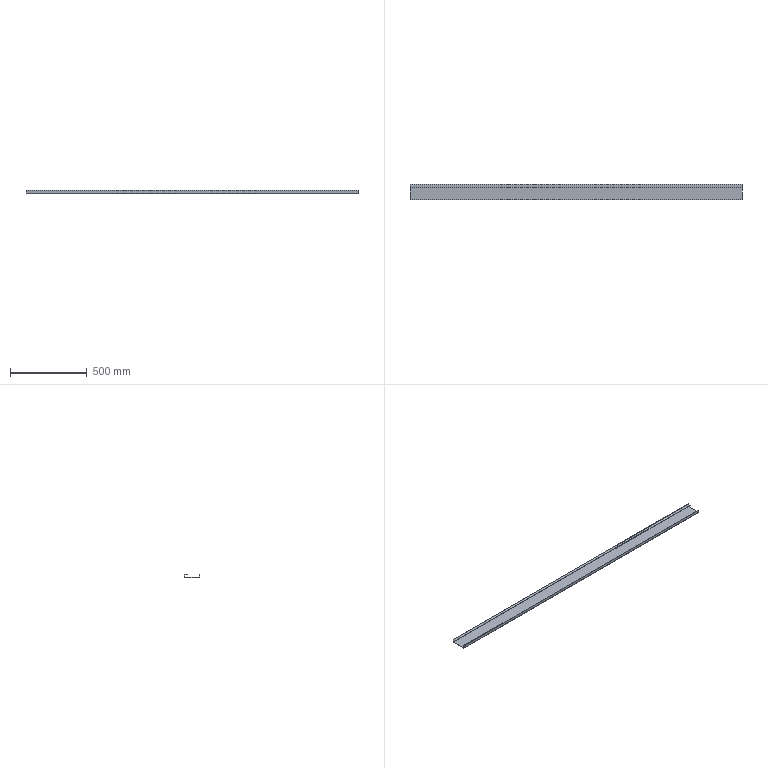Part | STEP file | 粉仓踢脚Plate 5 | 1 solid | 18 faces | box 2168 x 100 x 20 mm | volume 498243 mm3 | plane 12 | cylinder 6 | commonest cylinder face diameters 2 x3 5 x3
STEP:
#1=CARTESIAN_POINT('',(0.,0.,0.));
#2=DIRECTION('',(0.,0.,1.));
#3=DIRECTION('',(1.,0.,0.));
#4=AXIS2_PLACEMENT_3D('',#1,#2,#3);
#5=CARTESIAN_POINT('',(-1083.75,1.5,2.5));
#6=VERTEX_POINT('',#5);
#7=CARTESIAN_POINT('',(-1083.75,1.5,20.));
#8=VERTEX_POINT('',#7);
#9=CARTESIAN_POINT('',(-1083.75,1.5,2.5));
#10=DIRECTION('',(0.,0.,1.));
#11=VECTOR('',#10,1.);
#12=LINE('',#9,#11);
#13=CARTESIAN_POINT('',(1083.75,1.5,2.5));
#14=DIRECTION('',(0.,-1.,0.));
#15=DIRECTION('',(0.,0.,-1.));
#16=AXIS2_PLACEMENT_3D('',#13,#14,#15);
#17=PLANE('',#16);
#18=CARTESIAN_POINT('',(0.,-2167.5));
#19=DIRECTION('',(-1.,0.));
#20=VECTOR('',#19,1.);
#21=LINE('',#18,#20);
#22=(GEOMETRIC_REPRESENTATION_CONTEXT(2)PARAMETRIC_REPRESENTATION_CONTEXT()REPRESENTATION_CONTEXT('',''));
#23=DEFINITIONAL_REPRESENTATION('',(#21),#22);
#24=PCURVE('',#17,#23);
#25=CARTESIAN_POINT('',(-1083.75,2.5,2.5));
#26=DIRECTION('',(-1.,0.,0.));
#27=DIRECTION('',(0.,0.,1.));
#28=AXIS2_PLACEMENT_3D('',#25,#26,#27);
#29=PLANE('',#28);
#30=CARTESIAN_POINT('',(0.,-1.));
#31=DIRECTION('',(1.,0.));
#32=VECTOR('',#31,1.);
#33=LINE('',#30,#32);
#34=(GEOMETRIC_REPRESENTATION_CONTEXT(2)PARAMETRIC_REPRESENTATION_CONTEXT()REPRESENTATION_CONTEXT('',''));
#35=DEFINITIONAL_REPRESENTATION('',(#33),#34);
#36=PCURVE('',#29,#35);
#37=SURFACE_CURVE('',#12,(#24,#36),.PCURVE_S1.);
#38=EDGE_CURVE('',#6,#8,#37,.T.);
#39=ORIENTED_EDGE('',*,*,#38,.T.);
#40=CARTESIAN_POINT('',(1083.75,1.5,20.));
#41=VERTEX_POINT('',#40);
#42=CARTESIAN_POINT('',(1083.75,1.5,20.));
#43=DIRECTION('',(-1.,0.,0.));
#44=VECTOR('',#43,1.);
#45=LINE('',#42,#44);
#46=CARTESIAN_POINT('',(-17.5,0.));
#47=DIRECTION('',(0.,-1.));
#48=VECTOR('',#47,1.);
#49=LINE('',#46,#48);
#50=(GEOMETRIC_REPRESENTATION_CONTEXT(2)PARAMETRIC_REPRESENTATION_CONTEXT()REPRESENTATION_CONTEXT('',''));
#51=DEFINITIONAL_REPRESENTATION('',(#49),#50);
#52=PCURVE('',#17,#51);
#53=CARTESIAN_POINT('',(1083.75,0.,20.));
#54=DIRECTION('',(0.,0.,1.));
#55=DIRECTION('',(1.,0.,0.));
#56=AXIS2_PLACEMENT_3D('',#53,#54,#55);
#57=PLANE('',#56);
#58=CARTESIAN_POINT('',(0.,1.5));
#59=DIRECTION('',(-1.,0.));
#60=VECTOR('',#59,1.);
#61=LINE('',#58,#60);
#62=(GEOMETRIC_REPRESENTATION_CONTEXT(2)PARAMETRIC_REPRESENTATION_CONTEXT()REPRESENTATION_CONTEXT('',''));
#63=DEFINITIONAL_REPRESENTATION('',(#61),#62);
#64=PCURVE('',#57,#63);
#65=SURFACE_CURVE('',#45,(#52,#64),.PCURVE_S1.);
#66=EDGE_CURVE('',#41,#8,#65,.T.);
#67=ORIENTED_EDGE('',*,*,#66,.F.);
#68=CARTESIAN_POINT('',(1083.75,1.5,2.5));
#69=VERTEX_POINT('',#68);
#70=CARTESIAN_POINT('',(1083.75,1.5,2.5));
#71=DIRECTION('',(0.,0.,1.));
#72=VECTOR('',#71,1.);
#73=LINE('',#70,#72);
#74=CARTESIAN_POINT('',(0.,0.));
#75=DIRECTION('',(-1.,0.));
#76=VECTOR('',#75,1.);
#77=LINE('',#74,#76);
#78=(GEOMETRIC_REPRESENTATION_CONTEXT(2)PARAMETRIC_REPRESENTATION_CONTEXT()REPRESENTATION_CONTEXT('',''));
#79=DEFINITIONAL_REPRESENTATION('',(#77),#78);
#80=PCURVE('',#17,#79);
#81=CARTESIAN_POINT('',(1083.75,2.5,2.5));
#82=DIRECTION('',(-1.,0.,0.));
#83=DIRECTION('',(0.,0.,1.));
#84=AXIS2_PLACEMENT_3D('',#81,#82,#83);
#85=PLANE('',#84);
#86=CARTESIAN_POINT('',(0.,-1.));
#87=DIRECTION('',(1.,0.));
#88=VECTOR('',#87,1.);
#89=LINE('',#86,#88);
#90=(GEOMETRIC_REPRESENTATION_CONTEXT(2)PARAMETRIC_REPRESENTATION_CONTEXT()REPRESENTATION_CONTEXT('',''));
#91=DEFINITIONAL_REPRESENTATION('',(#89),#90);
#92=PCURVE('',#85,#91);
#93=SURFACE_CURVE('',#73,(#80,#92),.PCURVE_S1.);
#94=EDGE_CURVE('',#69,#41,#93,.T.);
#95=ORIENTED_EDGE('',*,*,#94,.F.);
#96=CARTESIAN_POINT('',(1083.75,1.5,2.5));
#97=DIRECTION('',(-1.,0.,0.));
#98=VECTOR('',#97,1.);
#99=LINE('',#96,#98);
#100=CARTESIAN_POINT('',(0.,0.));
#101=DIRECTION('',(0.,-1.));
#102=VECTOR('',#101,1.);
#103=LINE('',#100,#102);
#104=(GEOMETRIC_REPRESENTATION_CONTEXT(2)PARAMETRIC_REPRESENTATION_CONTEXT()REPRESENTATION_CONTEXT('',''));
#105=DEFINITIONAL_REPRESENTATION('',(#103),#104);
#106=PCURVE('',#17,#105);
#107=CARTESIAN_POINT('',(1083.75,2.5,2.5));
#108=DIRECTION('',(-1.,0.,0.));
#109=DIRECTION('',(0.,0.,1.));
#110=AXIS2_PLACEMENT_3D('',#107,#108,#109);
#111=CYLINDRICAL_SURFACE('',#110,1.);
#112=CARTESIAN_POINT('',(4.712,0.));
#113=DIRECTION('',(0.,1.));
#114=VECTOR('',#113,1.);
#115=LINE('',#112,#114);
#116=(GEOMETRIC_REPRESENTATION_CONTEXT(2)PARAMETRIC_REPRESENTATION_CONTEXT()REPRESENTATION_CONTEXT('',''));
#117=DEFINITIONAL_REPRESENTATION('',(#115),#116);
#118=PCURVE('',#111,#117);
#119=SURFACE_CURVE('',#99,(#106,#118),.PCURVE_S1.);
#120=EDGE_CURVE('',#69,#6,#119,.T.);
#121=ORIENTED_EDGE('',*,*,#120,.T.);
#122=EDGE_LOOP('',(#39,#67,#95,#121));
#123=FACE_BOUND('',#122,.T.);
#124=ADVANCED_FACE('',(#123),#17,.F.);
#125=CARTESIAN_POINT('',(-1083.75,0.,20.));
#126=VERTEX_POINT('',#125);
#127=CARTESIAN_POINT('',(-1083.75,0.,20.));
#128=DIRECTION('',(0.,1.,0.));
#129=VECTOR('',#128,1.);
#130=LINE('',#127,#129);
#131=CARTESIAN_POINT('',(-2167.5,0.));
#132=DIRECTION('',(0.,1.));
#133=VECTOR('',#132,1.);
#134=LINE('',#131,#133);
#135=(GEOMETRIC_REPRESENTATION_CONTEXT(2)PARAMETRIC_REPRESENTATION_CONTEXT()REPRESENTATION_CONTEXT('',''));
#136=DEFINITIONAL_REPRESENTATION('',(#134),#135);
#137=PCURVE('',#57,#136);
#138=CARTESIAN_POINT('',(17.5,-2.5));
#139=DIRECTION('',(0.,1.));
#140=VECTOR('',#139,1.);
#141=LINE('',#138,#140);
#142=(GEOMETRIC_REPRESENTATION_CONTEXT(2)PARAMETRIC_REPRESENTATION_CONTEXT()REPRESENTATION_CONTEXT('',''));
#143=DEFINITIONAL_REPRESENTATION('',(#141),#142);
#144=PCURVE('',#29,#143);
#145=SURFACE_CURVE('',#130,(#137,#144),.PCURVE_S1.);
#146=EDGE_CURVE('',#126,#8,#145,.T.);
#147=ORIENTED_EDGE('',*,*,#146,.F.);
#148=CARTESIAN_POINT('',(1083.75,0.,20.));
#149=VERTEX_POINT('',#148);
#150=CARTESIAN_POINT('',(1083.75,0.,20.));
#151=DIRECTION('',(-1.,0.,0.));
#152=VECTOR('',#151,1.);
#153=LINE('',#150,#152);
#154=CARTESIAN_POINT('',(0.,0.));
#155=DIRECTION('',(-1.,0.));
#156=VECTOR('',#155,1.);
#157=LINE('',#154,#156);
#158=(GEOMETRIC_REPRESENTATION_CONTEXT(2)PARAMETRIC_REPRESENTATION_CONTEXT()REPRESENTATION_CONTEXT('',''));
#159=DEFINITIONAL_REPRESENTATION('',(#157),#158);
#160=PCURVE('',#57,#159);
#161=CARTESIAN_POINT('',(1083.75,0.,2.5));
#162=DIRECTION('',(0.,-1.,0.));
#163=DIRECTION('',(0.,0.,-1.));
#164=AXIS2_PLACEMENT_3D('',#161,#162,#163);
#165=PLANE('',#164);
#166=CARTESIAN_POINT('',(-17.5,0.));
#167=DIRECTION('',(0.,-1.));
#168=VECTOR('',#167,1.);
#169=LINE('',#166,#168);
#170=(GEOMETRIC_REPRESENTATION_CONTEXT(2)PARAMETRIC_REPRESENTATION_CONTEXT()REPRESENTATION_CONTEXT('',''));
#171=DEFINITIONAL_REPRESENTATION('',(#169),#170);
#172=PCURVE('',#165,#171);
#173=SURFACE_CURVE('',#153,(#160,#172),.PCURVE_S1.);
#174=EDGE_CURVE('',#149,#126,#173,.T.);
#175=ORIENTED_EDGE('',*,*,#174,.F.);
#176=CARTESIAN_POINT('',(1083.75,0.,20.));
#177=DIRECTION('',(0.,1.,0.));
#178=VECTOR('',#177,1.);
#179=LINE('',#176,#178);
#180=CARTESIAN_POINT('',(0.,0.));
#181=DIRECTION('',(0.,1.));
#182=VECTOR('',#181,1.);
#183=LINE('',#180,#182);
#184=(GEOMETRIC_REPRESENTATION_CONTEXT(2)PARAMETRIC_REPRESENTATION_CONTEXT()REPRESENTATION_CONTEXT('',''));
#185=DEFINITIONAL_REPRESENTATION('',(#183),#184);
#186=PCURVE('',#57,#185);
#187=CARTESIAN_POINT('',(17.5,-2.5));
#188=DIRECTION('',(0.,1.));
#189=VECTOR('',#188,1.);
#190=LINE('',#187,#189);
#191=(GEOMETRIC_REPRESENTATION_CONTEXT(2)PARAMETRIC_REPRESENTATION_CONTEXT()REPRESENTATION_CONTEXT('',''));
#192=DEFINITIONAL_REPRESENTATION('',(#190),#191);
#193=PCURVE('',#85,#192);
#194=SURFACE_CURVE('',#179,(#186,#193),.PCURVE_S1.);
#195=EDGE_CURVE('',#149,#41,#194,.T.);
#196=ORIENTED_EDGE('',*,*,#195,.T.);
#197=ORIENTED_EDGE('',*,*,#66,.T.);
#198=EDGE_LOOP('',(#147,#175,#196,#197));
#199=FACE_BOUND('',#198,.T.);
#200=ADVANCED_FACE('',(#199),#57,.T.);
#201=CARTESIAN_POINT('',(-1083.75,0.,2.5));
#202=VERTEX_POINT('',#201);
#203=CARTESIAN_POINT('',(-1083.75,0.,2.5));
#204=DIRECTION('',(0.,0.,1.));
#205=VECTOR('',#204,1.);
#206=LINE('',#203,#205);
#207=CARTESIAN_POINT('',(0.,-2167.5));
#208=DIRECTION('',(-1.,0.));
#209=VECTOR('',#208,1.);
#210=LINE('',#207,#209);
#211=(GEOMETRIC_REPRESENTATION_CONTEXT(2)PARAMETRIC_REPRESENTATION_CONTEXT()REPRESENTATION_CONTEXT('',''));
#212=DEFINITIONAL_REPRESENTATION('',(#210),#211);
#213=PCURVE('',#165,#212);
#214=CARTESIAN_POINT('',(0.,-2.5));
#215=DIRECTION('',(1.,0.));
#216=VECTOR('',#215,1.);
#217=LINE('',#214,#216);
#218=(GEOMETRIC_REPRESENTATION_CONTEXT(2)PARAMETRIC_REPRESENTATION_CONTEXT()REPRESENTATION_CONTEXT('',''));
#219=DEFINITIONAL_REPRESENTATION('',(#217),#218);
#220=PCURVE('',#29,#219);
#221=SURFACE_CURVE('',#206,(#213,#220),.PCURVE_S1.);
#222=EDGE_CURVE('',#202,#126,#221,.T.);
#223=ORIENTED_EDGE('',*,*,#222,.F.);
#224=CARTESIAN_POINT('',(1083.75,0.,2.5));
#225=VERTEX_POINT('',#224);
#226=CARTESIAN_POINT('',(1083.75,0.,2.5));
#227=DIRECTION('',(-1.,0.,0.));
#228=VECTOR('',#227,1.);
#229=LINE('',#226,#228);
#230=CARTESIAN_POINT('',(0.,0.));
#231=DIRECTION('',(0.,-1.));
#232=VECTOR('',#231,1.);
#233=LINE('',#230,#232);
#234=(GEOMETRIC_REPRESENTATION_CONTEXT(2)PARAMETRIC_REPRESENTATION_CONTEXT()REPRESENTATION_CONTEXT('',''));
#235=DEFINITIONAL_REPRESENTATION('',(#233),#234);
#236=PCURVE('',#165,#235);
#237=CARTESIAN_POINT('',(1083.75,2.5,2.5));
#238=DIRECTION('',(-1.,0.,0.));
#239=DIRECTION('',(0.,0.,1.));
#240=AXIS2_PLACEMENT_3D('',#237,#238,#239);
#241=CYLINDRICAL_SURFACE('',#240,2.5);
#242=CARTESIAN_POINT('',(4.712,0.));
#243=DIRECTION('',(0.,1.));
#244=VECTOR('',#243,1.);
#245=LINE('',#242,#244);
#246=(GEOMETRIC_REPRESENTATION_CONTEXT(2)PARAMETRIC_REPRESENTATION_CONTEXT()REPRESENTATION_CONTEXT('',''));
#247=DEFINITIONAL_REPRESENTATION('',(#245),#246);
#248=PCURVE('',#241,#247);
#249=SURFACE_CURVE('',#229,(#236,#248),.PCURVE_S1.);
#250=EDGE_CURVE('',#225,#202,#249,.T.);
#251=ORIENTED_EDGE('',*,*,#250,.F.);
#252=CARTESIAN_POINT('',(1083.75,0.,2.5));
#253=DIRECTION('',(0.,0.,1.));
#254=VECTOR('',#253,1.);
#255=LINE('',#252,#254);
#256=CARTESIAN_POINT('',(0.,0.));
#257=DIRECTION('',(-1.,0.));
#258=VECTOR('',#257,1.);
#259=LINE('',#256,#258);
#260=(GEOMETRIC_REPRESENTATION_CONTEXT(2)PARAMETRIC_REPRESENTATION_CONTEXT()REPRESENTATION_CONTEXT('',''));
#261=DEFINITIONAL_REPRESENTATION('',(#259),#260);
#262=PCURVE('',#165,#261);
#263=CARTESIAN_POINT('',(0.,-2.5));
#264=DIRECTION('',(1.,0.));
#265=VECTOR('',#264,1.);
#266=LINE('',#263,#265);
#267=(GEOMETRIC_REPRESENTATION_CONTEXT(2)PARAMETRIC_REPRESENTATION_CONTEXT()REPRESENTATION_CONTEXT('',''));
#268=DEFINITIONAL_REPRESENTATION('',(#266),#267);
#269=PCURVE('',#85,#268);
#270=SURFACE_CURVE('',#255,(#262,#269),.PCURVE_S1.);
#271=EDGE_CURVE('',#225,#149,#270,.T.);
#272=ORIENTED_EDGE('',*,*,#271,.T.);
#273=ORIENTED_EDGE('',*,*,#174,.T.);
#274=EDGE_LOOP('',(#223,#251,#272,#273));
#275=FACE_BOUND('',#274,.T.);
#276=ADVANCED_FACE('',(#275),#165,.T.);
#277=CARTESIAN_POINT('',(-1083.75,2.5,0.));
#278=VERTEX_POINT('',#277);
#279=CARTESIAN_POINT('',(-1083.75,2.5,2.5));
#280=DIRECTION('',(-1.,0.,0.));
#281=DIRECTION('',(0.,0.,1.));
#282=AXIS2_PLACEMENT_3D('',#279,#280,#281);
#283=CIRCLE('',#282,2.5);
#284=CARTESIAN_POINT('',(0.,2167.5));
#285=DIRECTION('',(1.,0.));
#286=VECTOR('',#285,1.);
#287=LINE('',#284,#286);
#288=(GEOMETRIC_REPRESENTATION_CONTEXT(2)PARAMETRIC_REPRESENTATION_CONTEXT()REPRESENTATION_CONTEXT('',''));
#289=DEFINITIONAL_REPRESENTATION('',(#287),#288);
#290=PCURVE('',#241,#289);
#291=CARTESIAN_POINT('',(0.,0.));
#292=DIRECTION('',(1.,0.));
#293=AXIS2_PLACEMENT_2D('',#291,#292);
#294=CIRCLE('',#293,2.5);
#295=(GEOMETRIC_REPRESENTATION_CONTEXT(2)PARAMETRIC_REPRESENTATION_CONTEXT()REPRESENTATION_CONTEXT('',''));
#296=DEFINITIONAL_REPRESENTATION('',(#294),#295);
#297=PCURVE('',#29,#296);
#298=SURFACE_CURVE('',#283,(#290,#297),.PCURVE_S1.);
#299=EDGE_CURVE('',#278,#202,#298,.T.);
#300=ORIENTED_EDGE('',*,*,#299,.F.);
#301=CARTESIAN_POINT('',(1083.75,2.5,0.));
#302=VERTEX_POINT('',#301);
#303=CARTESIAN_POINT('',(1083.75,2.5,0.));
#304=DIRECTION('',(-1.,0.,0.));
#305=VECTOR('',#304,1.);
#306=LINE('',#303,#305);
#307=CARTESIAN_POINT('',(3.142,0.));
#308=DIRECTION('',(0.,1.));
#309=VECTOR('',#308,1.);
#310=LINE('',#307,#309);
#311=(GEOMETRIC_REPRESENTATION_CONTEXT(2)PARAMETRIC_REPRESENTATION_CONTEXT()REPRESENTATION_CONTEXT('',''));
#312=DEFINITIONAL_REPRESENTATION('',(#310),#311);
#313=PCURVE('',#241,#312);
#314=CARTESIAN_POINT('',(1083.75,2.5,0.));
#315=DIRECTION('',(0.,0.,-1.));
#316=DIRECTION('',(-1.,0.,0.));
#317=AXIS2_PLACEMENT_3D('',#314,#315,#316);
#318=PLANE('',#317);
#319=CARTESIAN_POINT('',(0.,0.));
#320=DIRECTION('',(1.,0.));
#321=VECTOR('',#320,1.);
#322=LINE('',#319,#321);
#323=(GEOMETRIC_REPRESENTATION_CONTEXT(2)PARAMETRIC_REPRESENTATION_CONTEXT()REPRESENTATION_CONTEXT('',''));
#324=DEFINITIONAL_REPRESENTATION('',(#322),#323);
#325=PCURVE('',#318,#324);
#326=SURFACE_CURVE('',#306,(#313,#325),.PCURVE_S1.);
#327=EDGE_CURVE('',#302,#278,#326,.T.);
#328=ORIENTED_EDGE('',*,*,#327,.F.);
#329=CARTESIAN_POINT('',(1083.75,2.5,2.5));
#330=DIRECTION('',(-1.,0.,0.));
#331=DIRECTION('',(0.,0.,1.));
#332=AXIS2_PLACEMENT_3D('',#329,#330,#331);
#333=CIRCLE('',#332,2.5);
#334=CARTESIAN_POINT('',(0.,0.));
#335=DIRECTION('',(1.,0.));
#336=VECTOR('',#335,1.);
#337=LINE('',#334,#336);
#338=(GEOMETRIC_REPRESENTATION_CONTEXT(2)PARAMETRIC_REPRESENTATION_CONTEXT()REPRESENTATION_CONTEXT('',''));
#339=DEFINITIONAL_REPRESENTATION('',(#337),#338);
#340=PCURVE('',#241,#339);
#341=CARTESIAN_POINT('',(0.,0.));
#342=DIRECTION('',(1.,0.));
#343=AXIS2_PLACEMENT_2D('',#341,#342);
#344=CIRCLE('',#343,2.5);
#345=(GEOMETRIC_REPRESENTATION_CONTEXT(2)PARAMETRIC_REPRESENTATION_CONTEXT()REPRESENTATION_CONTEXT('',''));
#346=DEFINITIONAL_REPRESENTATION('',(#344),#345);
#347=PCURVE('',#85,#346);
#348=SURFACE_CURVE('',#333,(#340,#347),.PCURVE_S1.);
#349=EDGE_CURVE('',#302,#225,#348,.T.);
#350=ORIENTED_EDGE('',*,*,#349,.T.);
#351=ORIENTED_EDGE('',*,*,#250,.T.);
#352=EDGE_LOOP('',(#300,#328,#350,#351));
#353=FACE_BOUND('',#352,.T.);
#354=ADVANCED_FACE('',(#353),#241,.T.);
#355=CARTESIAN_POINT('',(-1083.75,97.5,0.));
#356=VERTEX_POINT('',#355);
#357=CARTESIAN_POINT('',(-1083.75,2.5,0.));
#358=DIRECTION('',(0.,-1.,0.));
#359=VECTOR('',#358,1.);
#360=LINE('',#357,#359);
#361=CARTESIAN_POINT('',(2167.5,0.));
#362=DIRECTION('',(0.,-1.));
#363=VECTOR('',#362,1.);
#364=LINE('',#361,#363);
#365=(GEOMETRIC_REPRESENTATION_CONTEXT(2)PARAMETRIC_REPRESENTATION_CONTEXT()REPRESENTATION_CONTEXT('',''));
#366=DEFINITIONAL_REPRESENTATION('',(#364),#365);
#367=PCURVE('',#318,#366);
#368=CARTESIAN_POINT('',(-2.5,0.));
#369=DIRECTION('',(0.,-1.));
#370=VECTOR('',#369,1.);
#371=LINE('',#368,#370);
#372=(GEOMETRIC_REPRESENTATION_CONTEXT(2)PARAMETRIC_REPRESENTATION_CONTEXT()REPRESENTATION_CONTEXT('',''));
#373=DEFINITIONAL_REPRESENTATION('',(#371),#372);
#374=PCURVE('',#29,#373);
#375=SURFACE_CURVE('',#360,(#367,#374),.PCURVE_S1.);
#376=EDGE_CURVE('',#356,#278,#375,.T.);
#377=ORIENTED_EDGE('',*,*,#376,.F.);
#378=CARTESIAN_POINT('',(1083.75,97.5,0.));
#379=VERTEX_POINT('',#378);
#380=CARTESIAN_POINT('',(1083.75,97.5,0.));
#381=DIRECTION('',(-1.,0.,0.));
#382=VECTOR('',#381,1.);
#383=LINE('',#380,#382);
#384=CARTESIAN_POINT('',(0.,95.));
#385=DIRECTION('',(1.,0.));
#386=VECTOR('',#385,1.);
#387=LINE('',#384,#386);
#388=(GEOMETRIC_REPRESENTATION_CONTEXT(2)PARAMETRIC_REPRESENTATION_CONTEXT()REPRESENTATION_CONTEXT('',''));
#389=DEFINITIONAL_REPRESENTATION('',(#387),#388);
#390=PCURVE('',#318,#389);
#391=CARTESIAN_POINT('',(1083.75,97.5,2.5));
#392=DIRECTION('',(-1.,0.,0.));
#393=DIRECTION('',(0.,0.,1.));
#394=AXIS2_PLACEMENT_3D('',#391,#392,#393);
#395=CYLINDRICAL_SURFACE('',#394,2.5);
#396=CARTESIAN_POINT('',(3.142,0.));
#397=DIRECTION('',(0.,1.));
#398=VECTOR('',#397,1.);
#399=LINE('',#396,#398);
#400=(GEOMETRIC_REPRESENTATION_CONTEXT(2)PARAMETRIC_REPRESENTATION_CONTEXT()REPRESENTATION_CONTEXT('',''));
#401=DEFINITIONAL_REPRESENTATION('',(#399),#400);
#402=PCURVE('',#395,#401);
#403=SURFACE_CURVE('',#383,(#390,#402),.PCURVE_S1.);
#404=EDGE_CURVE('',#379,#356,#403,.T.);
#405=ORIENTED_EDGE('',*,*,#404,.F.);
#406=CARTESIAN_POINT('',(1083.75,2.5,0.));
#407=DIRECTION('',(0.,-1.,0.));
#408=VECTOR('',#407,1.);
#409=LINE('',#406,#408);
#410=CARTESIAN_POINT('',(0.,0.));
#411=DIRECTION('',(0.,-1.));
#412=VECTOR('',#411,1.);
#413=LINE('',#410,#412);
#414=(GEOMETRIC_REPRESENTATION_CONTEXT(2)PARAMETRIC_REPRESENTATION_CONTEXT()REPRESENTATION_CONTEXT('',''));
#415=DEFINITIONAL_REPRESENTATION('',(#413),#414);
#416=PCURVE('',#318,#415);
#417=CARTESIAN_POINT('',(-2.5,0.));
#418=DIRECTION('',(0.,-1.));
#419=VECTOR('',#418,1.);
#420=LINE('',#417,#419);
#421=(GEOMETRIC_REPRESENTATION_CONTEXT(2)PARAMETRIC_REPRESENTATION_CONTEXT()REPRESENTATION_CONTEXT('',''));
#422=DEFINITIONAL_REPRESENTATION('',(#420),#421);
#423=PCURVE('',#85,#422);
#424=SURFACE_CURVE('',#409,(#416,#423),.PCURVE_S1.);
#425=EDGE_CURVE('',#379,#302,#424,.T.);
#426=ORIENTED_EDGE('',*,*,#425,.T.);
#427=ORIENTED_EDGE('',*,*,#327,.T.);
#428=EDGE_LOOP('',(#377,#405,#426,#427));
#429=FACE_BOUND('',#428,.T.);
#430=ADVANCED_FACE('',(#429),#318,.T.);
#431=CARTESIAN_POINT('',(-1083.75,100.,2.5));
#432=VERTEX_POINT('',#431);
#433=CARTESIAN_POINT('',(-1083.75,97.5,2.5));
#434=DIRECTION('',(-1.,0.,0.));
#435=DIRECTION('',(0.,0.,-1.));
#436=AXIS2_PLACEMENT_3D('',#433,#434,#435);
#437=CIRCLE('',#436,2.5);
#438=CARTESIAN_POINT('',(-3.142,2167.5));
#439=DIRECTION('',(1.,0.));
#440=VECTOR('',#439,1.);
#441=LINE('',#438,#440);
#442=(GEOMETRIC_REPRESENTATION_CONTEXT(2)PARAMETRIC_REPRESENTATION_CONTEXT()REPRESENTATION_CONTEXT('',''));
#443=DEFINITIONAL_REPRESENTATION('',(#441),#442);
#444=PCURVE('',#395,#443);
#445=CARTESIAN_POINT('',(0.,95.));
#446=DIRECTION('',(-1.,0.));
#447=AXIS2_PLACEMENT_2D('',#445,#446);
#448=CIRCLE('',#447,2.5);
#449=(GEOMETRIC_REPRESENTATION_CONTEXT(2)PARAMETRIC_REPRESENTATION_CONTEXT()REPRESENTATION_CONTEXT('',''));
#450=DEFINITIONAL_REPRESENTATION('',(#448),#449);
#451=PCURVE('',#29,#450);
#452=SURFACE_CURVE('',#437,(#444,#451),.PCURVE_S1.);
#453=EDGE_CURVE('',#432,#356,#452,.T.);
#454=ORIENTED_EDGE('',*,*,#453,.F.);
#455=CARTESIAN_POINT('',(1083.75,100.,2.5));
#456=VERTEX_POINT('',#455);
#457=CARTESIAN_POINT('',(1083.75,100.,2.5));
#458=DIRECTION('',(-1.,0.,0.));
#459=VECTOR('',#458,1.);
#460=LINE('',#457,#459);
#461=CARTESIAN_POINT('',(1.571,0.));
#462=DIRECTION('',(0.,1.));
#463=VECTOR('',#462,1.);
#464=LINE('',#461,#463);
#465=(GEOMETRIC_REPRESENTATION_CONTEXT(2)PARAMETRIC_REPRESENTATION_CONTEXT()REPRESENTATION_CONTEXT('',''));
#466=DEFINITIONAL_REPRESENTATION('',(#464),#465);
#467=PCURVE('',#395,#466);
#468=CARTESIAN_POINT('',(1083.75,100.,2.5));
#469=DIRECTION('',(0.,1.,0.));
#470=DIRECTION('',(0.,0.,1.));
#471=AXIS2_PLACEMENT_3D('',#468,#469,#470);
#472=PLANE('',#471);
#473=CARTESIAN_POINT('',(0.,0.));
#474=DIRECTION('',(0.,-1.));
#475=VECTOR('',#474,1.);
#476=LINE('',#473,#475);
#477=(GEOMETRIC_REPRESENTATION_CONTEXT(2)PARAMETRIC_REPRESENTATION_CONTEXT()REPRESENTATION_CONTEXT('',''));
#478=DEFINITIONAL_REPRESENTATION('',(#476),#477);
#479=PCURVE('',#472,#478);
#480=SURFACE_CURVE('',#460,(#467,#479),.PCURVE_S1.);
#481=EDGE_CURVE('',#456,#432,#480,.T.);
#482=ORIENTED_EDGE('',*,*,#481,.F.);
#483=CARTESIAN_POINT('',(1083.75,97.5,2.5));
#484=DIRECTION('',(-1.,0.,0.));
#485=DIRECTION('',(0.,0.,-1.));
#486=AXIS2_PLACEMENT_3D('',#483,#484,#485);
#487=CIRCLE('',#486,2.5);
#488=CARTESIAN_POINT('',(-3.142,0.));
#489=DIRECTION('',(1.,0.));
#490=VECTOR('',#489,1.);
#491=LINE('',#488,#490);
#492=(GEOMETRIC_REPRESENTATION_CONTEXT(2)PARAMETRIC_REPRESENTATION_CONTEXT()REPRESENTATION_CONTEXT('',''));
#493=DEFINITIONAL_REPRESENTATION('',(#491),#492);
#494=PCURVE('',#395,#493);
#495=CARTESIAN_POINT('',(0.,95.));
#496=DIRECTION('',(-1.,0.));
#497=AXIS2_PLACEMENT_2D('',#495,#496);
#498=CIRCLE('',#497,2.5);
#499=(GEOMETRIC_REPRESENTATION_CONTEXT(2)PARAMETRIC_REPRESENTATION_CONTEXT()REPRESENTATION_CONTEXT('',''));
#500=DEFINITIONAL_REPRESENTATION('',(#498),#499);
#501=PCURVE('',#85,#500);
#502=SURFACE_CURVE('',#487,(#494,#501),.PCURVE_S1.);
#503=EDGE_CURVE('',#456,#379,#502,.T.);
#504=ORIENTED_EDGE('',*,*,#503,.T.);
#505=ORIENTED_EDGE('',*,*,#404,.T.);
#506=EDGE_LOOP('',(#454,#482,#504,#505));
#507=FACE_BOUND('',#506,.T.);
#508=ADVANCED_FACE('',(#507),#395,.T.);
#509=CARTESIAN_POINT('',(-1083.75,100.,17.5));
#510=VERTEX_POINT('',#509);
#511=CARTESIAN_POINT('',(-1083.75,100.,2.5));
#512=DIRECTION('',(0.,0.,-1.));
#513=VECTOR('',#512,1.);
#514=LINE('',#511,#513);
#515=CARTESIAN_POINT('',(0.,-2167.5));
#516=DIRECTION('',(-1.,0.));
#517=VECTOR('',#516,1.);
#518=LINE('',#515,#517);
#519=(GEOMETRIC_REPRESENTATION_CONTEXT(2)PARAMETRIC_REPRESENTATION_CONTEXT()REPRESENTATION_CONTEXT('',''));
#520=DEFINITIONAL_REPRESENTATION('',(#518),#519);
#521=PCURVE('',#472,#520);
#522=CARTESIAN_POINT('',(0.,97.5));
#523=DIRECTION('',(-1.,0.));
#524=VECTOR('',#523,1.);
#525=LINE('',#522,#524);
#526=(GEOMETRIC_REPRESENTATION_CONTEXT(2)PARAMETRIC_REPRESENTATION_CONTEXT()REPRESENTATION_CONTEXT('',''));
#527=DEFINITIONAL_REPRESENTATION('',(#525),#526);
#528=PCURVE('',#29,#527);
#529=SURFACE_CURVE('',#514,(#521,#528),.PCURVE_S1.);
#530=EDGE_CURVE('',#510,#432,#529,.T.);
#531=ORIENTED_EDGE('',*,*,#530,.F.);
#532=CARTESIAN_POINT('',(1083.75,100.,17.5));
#533=VERTEX_POINT('',#532);
#534=CARTESIAN_POINT('',(1083.75,100.,17.5));
#535=DIRECTION('',(-1.,0.,0.));
#536=VECTOR('',#535,1.);
#537=LINE('',#534,#536);
#538=CARTESIAN_POINT('',(15.,0.));
#539=DIRECTION('',(0.,-1.));
#540=VECTOR('',#539,1.);
#541=LINE('',#538,#540);
#542=(GEOMETRIC_REPRESENTATION_CONTEXT(2)PARAMETRIC_REPRESENTATION_CONTEXT()REPRESENTATION_CONTEXT('',''));
#543=DEFINITIONAL_REPRESENTATION('',(#541),#542);
#544=PCURVE('',#472,#543);
#545=CARTESIAN_POINT('',(1083.75,97.5,17.5));
#546=DIRECTION('',(-1.,0.,0.));
#547=DIRECTION('',(0.,0.,1.));
#548=AXIS2_PLACEMENT_3D('',#545,#546,#547);
#549=CYLINDRICAL_SURFACE('',#548,2.5);
#550=CARTESIAN_POINT('',(1.571,0.));
#551=DIRECTION('',(0.,1.));
#552=VECTOR('',#551,1.);
#553=LINE('',#550,#552);
#554=(GEOMETRIC_REPRESENTATION_CONTEXT(2)PARAMETRIC_REPRESENTATION_CONTEXT()REPRESENTATION_CONTEXT('',''));
#555=DEFINITIONAL_REPRESENTATION('',(#553),#554);
#556=PCURVE('',#549,#555);
#557=SURFACE_CURVE('',#537,(#544,#556),.PCURVE_S1.);
#558=EDGE_CURVE('',#533,#510,#557,.T.);
#559=ORIENTED_EDGE('',*,*,#558,.F.);
#560=CARTESIAN_POINT('',(1083.75,100.,2.5));
#561=DIRECTION('',(0.,0.,-1.));
#562=VECTOR('',#561,1.);
#563=LINE('',#560,#562);
#564=CARTESIAN_POINT('',(0.,0.));
#565=DIRECTION('',(-1.,0.));
#566=VECTOR('',#565,1.);
#567=LINE('',#564,#566);
#568=(GEOMETRIC_REPRESENTATION_CONTEXT(2)PARAMETRIC_REPRESENTATION_CONTEXT()REPRESENTATION_CONTEXT('',''));
#569=DEFINITIONAL_REPRESENTATION('',(#567),#568);
#570=PCURVE('',#472,#569);
#571=CARTESIAN_POINT('',(0.,97.5));
#572=DIRECTION('',(-1.,0.));
#573=VECTOR('',#572,1.);
#574=LINE('',#571,#573);
#575=(GEOMETRIC_REPRESENTATION_CONTEXT(2)PARAMETRIC_REPRESENTATION_CONTEXT()REPRESENTATION_CONTEXT('',''));
#576=DEFINITIONAL_REPRESENTATION('',(#574),#575);
#577=PCURVE('',#85,#576);
#578=SURFACE_CURVE('',#563,(#570,#577),.PCURVE_S1.);
#579=EDGE_CURVE('',#533,#456,#578,.T.);
#580=ORIENTED_EDGE('',*,*,#579,.T.);
#581=ORIENTED_EDGE('',*,*,#481,.T.);
#582=EDGE_LOOP('',(#531,#559,#580,#581));
#583=FACE_BOUND('',#582,.T.);
#584=ADVANCED_FACE('',(#583),#472,.T.);
#585=CARTESIAN_POINT('',(-1083.75,97.5,20.));
#586=VERTEX_POINT('',#585);
#587=CARTESIAN_POINT('',(-1083.75,97.5,17.5));
#588=DIRECTION('',(-1.,0.,0.));
#589=DIRECTION('',(0.,0.,-1.));
#590=AXIS2_PLACEMENT_3D('',#587,#588,#589);
#591=CIRCLE('',#590,2.5);
#592=CARTESIAN_POINT('',(-3.142,2167.5));
#593=DIRECTION('',(1.,0.));
#594=VECTOR('',#593,1.);
#595=LINE('',#592,#594);
#596=(GEOMETRIC_REPRESENTATION_CONTEXT(2)PARAMETRIC_REPRESENTATION_CONTEXT()REPRESENTATION_CONTEXT('',''));
#597=DEFINITIONAL_REPRESENTATION('',(#595),#596);
#598=PCURVE('',#549,#597);
#599=CARTESIAN_POINT('',(15.,95.));
#600=DIRECTION('',(-1.,0.));
#601=AXIS2_PLACEMENT_2D('',#599,#600);
#602=CIRCLE('',#601,2.5);
#603=(GEOMETRIC_REPRESENTATION_CONTEXT(2)PARAMETRIC_REPRESENTATION_CONTEXT()REPRESENTATION_CONTEXT('',''));
#604=DEFINITIONAL_REPRESENTATION('',(#602),#603);
#605=PCURVE('',#29,#604);
#606=SURFACE_CURVE('',#591,(#598,#605),.PCURVE_S1.);
#607=EDGE_CURVE('',#586,#510,#606,.T.);
#608=ORIENTED_EDGE('',*,*,#607,.F.);
#609=CARTESIAN_POINT('',(1083.75,97.5,20.));
#610=VERTEX_POINT('',#609);
#611=CARTESIAN_POINT('',(1083.75,97.5,20.));
#612=DIRECTION('',(-1.,0.,0.));
#613=VECTOR('',#612,1.);
#614=LINE('',#611,#613);
#615=CARTESIAN_POINT('',(0.,0.));
#616=DIRECTION('',(0.,1.));
#617=VECTOR('',#616,1.);
#618=LINE('',#615,#617);
#619=(GEOMETRIC_REPRESENTATION_CONTEXT(2)PARAMETRIC_REPRESENTATION_CONTEXT()REPRESENTATION_CONTEXT('',''));
#620=DEFINITIONAL_REPRESENTATION('',(#618),#619);
#621=PCURVE('',#549,#620);
#622=CARTESIAN_POINT('',(1083.75,97.5,20.));
#623=DIRECTION('',(0.,0.,1.));
#624=DIRECTION('',(1.,0.,0.));
#625=AXIS2_PLACEMENT_3D('',#622,#623,#624);
#626=PLANE('',#625);
#627=CARTESIAN_POINT('',(0.,0.));
#628=DIRECTION('',(-1.,0.));
#629=VECTOR('',#628,1.);
#630=LINE('',#627,#629);
#631=(GEOMETRIC_REPRESENTATION_CONTEXT(2)PARAMETRIC_REPRESENTATION_CONTEXT()REPRESENTATION_CONTEXT('',''));
#632=DEFINITIONAL_REPRESENTATION('',(#630),#631);
#633=PCURVE('',#626,#632);
#634=SURFACE_CURVE('',#614,(#621,#633),.PCURVE_S1.);
#635=EDGE_CURVE('',#610,#586,#634,.T.);
#636=ORIENTED_EDGE('',*,*,#635,.F.);
#637=CARTESIAN_POINT('',(1083.75,97.5,17.5));
#638=DIRECTION('',(-1.,0.,0.));
#639=DIRECTION('',(0.,0.,-1.));
#640=AXIS2_PLACEMENT_3D('',#637,#638,#639);
#641=CIRCLE('',#640,2.5);
#642=CARTESIAN_POINT('',(-3.142,0.));
#643=DIRECTION('',(1.,0.));
#644=VECTOR('',#643,1.);
#645=LINE('',#642,#644);
#646=(GEOMETRIC_REPRESENTATION_CONTEXT(2)PARAMETRIC_REPRESENTATION_CONTEXT()REPRESENTATION_CONTEXT('',''));
#647=DEFINITIONAL_REPRESENTATION('',(#645),#646);
#648=PCURVE('',#549,#647);
#649=CARTESIAN_POINT('',(15.,95.));
#650=DIRECTION('',(-1.,0.));
#651=AXIS2_PLACEMENT_2D('',#649,#650);
#652=CIRCLE('',#651,2.5);
#653=(GEOMETRIC_REPRESENTATION_CONTEXT(2)PARAMETRIC_REPRESENTATION_CONTEXT()REPRESENTATION_CONTEXT('',''));
#654=DEFINITIONAL_REPRESENTATION('',(#652),#653);
#655=PCURVE('',#85,#654);
#656=SURFACE_CURVE('',#641,(#648,#655),.PCURVE_S1.);
#657=EDGE_CURVE('',#610,#533,#656,.T.);
#658=ORIENTED_EDGE('',*,*,#657,.T.);
#659=ORIENTED_EDGE('',*,*,#558,.T.);
#660=EDGE_LOOP('',(#608,#636,#658,#659));
#661=FACE_BOUND('',#660,.T.);
#662=ADVANCED_FACE('',(#661),#549,.T.);
#663=CARTESIAN_POINT('',(-1083.75,80.,20.));
#664=VERTEX_POINT('',#663);
#665=CARTESIAN_POINT('',(-1083.75,97.5,20.));
#666=DIRECTION('',(0.,1.,0.));
#667=VECTOR('',#666,1.);
#668=LINE('',#665,#667);
#669=CARTESIAN_POINT('',(-2167.5,0.));
#670=DIRECTION('',(0.,1.));
#671=VECTOR('',#670,1.);
#672=LINE('',#669,#671);
#673=(GEOMETRIC_REPRESENTATION_CONTEXT(2)PARAMETRIC_REPRESENTATION_CONTEXT()REPRESENTATION_CONTEXT('',''));
#674=DEFINITIONAL_REPRESENTATION('',(#672),#673);
#675=PCURVE('',#626,#674);
#676=CARTESIAN_POINT('',(17.5,95.));
#677=DIRECTION('',(0.,1.));
#678=VECTOR('',#677,1.);
#679=LINE('',#676,#678);
#680=(GEOMETRIC_REPRESENTATION_CONTEXT(2)PARAMETRIC_REPRESENTATION_CONTEXT()REPRESENTATION_CONTEXT('',''));
#681=DEFINITIONAL_REPRESENTATION('',(#679),#680);
#682=PCURVE('',#29,#681);
#683=SURFACE_CURVE('',#668,(#675,#682),.PCURVE_S1.);
#684=EDGE_CURVE('',#664,#586,#683,.T.);
#685=ORIENTED_EDGE('',*,*,#684,.F.);
#686=CARTESIAN_POINT('',(1083.75,80.,20.));
#687=VERTEX_POINT('',#686);
#688=CARTESIAN_POINT('',(1083.75,80.,20.));
#689=DIRECTION('',(-1.,0.,0.));
#690=VECTOR('',#689,1.);
#691=LINE('',#688,#690);
#692=CARTESIAN_POINT('',(0.,-17.5));
#693=DIRECTION('',(-1.,0.));
#694=VECTOR('',#693,1.);
#695=LINE('',#692,#694);
#696=(GEOMETRIC_REPRESENTATION_CONTEXT(2)PARAMETRIC_REPRESENTATION_CONTEXT()REPRESENTATION_CONTEXT('',''));
#697=DEFINITIONAL_REPRESENTATION('',(#695),#696);
#698=PCURVE('',#626,#697);
#699=CARTESIAN_POINT('',(1083.75,80.,18.5));
#700=DIRECTION('',(0.,-1.,0.));
#701=DIRECTION('',(0.,0.,-1.));
#702=AXIS2_PLACEMENT_3D('',#699,#700,#701);
#703=PLANE('',#702);
#704=CARTESIAN_POINT('',(-1.5,0.));
#705=DIRECTION('',(0.,-1.));
#706=VECTOR('',#705,1.);
#707=LINE('',#704,#706);
#708=(GEOMETRIC_REPRESENTATION_CONTEXT(2)PARAMETRIC_REPRESENTATION_CONTEXT()REPRESENTATION_CONTEXT('',''));
#709=DEFINITIONAL_REPRESENTATION('',(#707),#708);
#710=PCURVE('',#703,#709);
#711=SURFACE_CURVE('',#691,(#698,#710),.PCURVE_S1.);
#712=EDGE_CURVE('',#687,#664,#711,.T.);
#713=ORIENTED_EDGE('',*,*,#712,.F.);
#714=CARTESIAN_POINT('',(1083.75,97.5,20.));
#715=DIRECTION('',(0.,1.,0.));
#716=VECTOR('',#715,1.);
#717=LINE('',#714,#716);
#718=CARTESIAN_POINT('',(0.,0.));
#719=DIRECTION('',(0.,1.));
#720=VECTOR('',#719,1.);
#721=LINE('',#718,#720);
#722=(GEOMETRIC_REPRESENTATION_CONTEXT(2)PARAMETRIC_REPRESENTATION_CONTEXT()REPRESENTATION_CONTEXT('',''));
#723=DEFINITIONAL_REPRESENTATION('',(#721),#722);
#724=PCURVE('',#626,#723);
#725=CARTESIAN_POINT('',(17.5,95.));
#726=DIRECTION('',(0.,1.));
#727=VECTOR('',#726,1.);
#728=LINE('',#725,#727);
#729=(GEOMETRIC_REPRESENTATION_CONTEXT(2)PARAMETRIC_REPRESENTATION_CONTEXT()REPRESENTATION_CONTEXT('',''));
#730=DEFINITIONAL_REPRESENTATION('',(#728),#729);
#731=PCURVE('',#85,#730);
#732=SURFACE_CURVE('',#717,(#724,#731),.PCURVE_S1.);
#733=EDGE_CURVE('',#687,#610,#732,.T.);
#734=ORIENTED_EDGE('',*,*,#733,.T.);
#735=ORIENTED_EDGE('',*,*,#635,.T.);
#736=EDGE_LOOP('',(#685,#713,#734,#735));
#737=FACE_BOUND('',#736,.T.);
#738=ADVANCED_FACE('',(#737),#626,.T.);
#739=CARTESIAN_POINT('',(-1083.75,80.,18.5));
#740=VERTEX_POINT('',#739);
#741=CARTESIAN_POINT('',(-1083.75,80.,18.5));
#742=DIRECTION('',(0.,0.,1.));
#743=VECTOR('',#742,1.);
#744=LINE('',#741,#743);
#745=CARTESIAN_POINT('',(0.,-2167.5));
#746=DIRECTION('',(-1.,0.));
#747=VECTOR('',#746,1.);
#748=LINE('',#745,#747);
#749=(GEOMETRIC_REPRESENTATION_CONTEXT(2)PARAMETRIC_REPRESENTATION_CONTEXT()REPRESENTATION_CONTEXT('',''));
#750=DEFINITIONAL_REPRESENTATION('',(#748),#749);
#751=PCURVE('',#703,#750);
#752=CARTESIAN_POINT('',(16.,77.5));
#753=DIRECTION('',(1.,0.));
#754=VECTOR('',#753,1.);
#755=LINE('',#752,#754);
#756=(GEOMETRIC_REPRESENTATION_CONTEXT(2)PARAMETRIC_REPRESENTATION_CONTEXT()REPRESENTATION_CONTEXT('',''));
#757=DEFINITIONAL_REPRESENTATION('',(#755),#756);
#758=PCURVE('',#29,#757);
#759=SURFACE_CURVE('',#744,(#751,#758),.PCURVE_S1.);
#760=EDGE_CURVE('',#740,#664,#759,.T.);
#761=ORIENTED_EDGE('',*,*,#760,.F.);
#762=CARTESIAN_POINT('',(1083.75,80.,18.5));
#763=VERTEX_POINT('',#762);
#764=CARTESIAN_POINT('',(1083.75,80.,18.5));
#765=DIRECTION('',(-1.,0.,0.));
#766=VECTOR('',#765,1.);
#767=LINE('',#764,#766);
#768=CARTESIAN_POINT('',(0.,0.));
#769=DIRECTION('',(0.,-1.));
#770=VECTOR('',#769,1.);
#771=LINE('',#768,#770);
#772=(GEOMETRIC_REPRESENTATION_CONTEXT(2)PARAMETRIC_REPRESENTATION_CONTEXT()REPRESENTATION_CONTEXT('',''));
#773=DEFINITIONAL_REPRESENTATION('',(#771),#772);
#774=PCURVE('',#703,#773);
#775=CARTESIAN_POINT('',(1083.75,97.5,18.5));
#776=DIRECTION('',(0.,0.,1.));
#777=DIRECTION('',(1.,0.,0.));
#778=AXIS2_PLACEMENT_3D('',#775,#776,#777);
#779=PLANE('',#778);
#780=CARTESIAN_POINT('',(0.,-17.5));
#781=DIRECTION('',(-1.,0.));
#782=VECTOR('',#781,1.);
#783=LINE('',#780,#782);
#784=(GEOMETRIC_REPRESENTATION_CONTEXT(2)PARAMETRIC_REPRESENTATION_CONTEXT()REPRESENTATION_CONTEXT('',''));
#785=DEFINITIONAL_REPRESENTATION('',(#783),#784);
#786=PCURVE('',#779,#785);
#787=SURFACE_CURVE('',#767,(#774,#786),.PCURVE_S1.);
#788=EDGE_CURVE('',#763,#740,#787,.T.);
#789=ORIENTED_EDGE('',*,*,#788,.F.);
#790=CARTESIAN_POINT('',(1083.75,80.,18.5));
#791=DIRECTION('',(0.,0.,1.));
#792=VECTOR('',#791,1.);
#793=LINE('',#790,#792);
#794=CARTESIAN_POINT('',(0.,0.));
#795=DIRECTION('',(-1.,0.));
#796=VECTOR('',#795,1.);
#797=LINE('',#794,#796);
#798=(GEOMETRIC_REPRESENTATION_CONTEXT(2)PARAMETRIC_REPRESENTATION_CONTEXT()REPRESENTATION_CONTEXT('',''));
#799=DEFINITIONAL_REPRESENTATION('',(#797),#798);
#800=PCURVE('',#703,#799);
#801=CARTESIAN_POINT('',(16.,77.5));
#802=DIRECTION('',(1.,0.));
#803=VECTOR('',#802,1.);
#804=LINE('',#801,#803);
#805=(GEOMETRIC_REPRESENTATION_CONTEXT(2)PARAMETRIC_REPRESENTATION_CONTEXT()REPRESENTATION_CONTEXT('',''));
#806=DEFINITIONAL_REPRESENTATION('',(#804),#805);
#807=PCURVE('',#85,#806);
#808=SURFACE_CURVE('',#793,(#800,#807),.PCURVE_S1.);
#809=EDGE_CURVE('',#763,#687,#808,.T.);
#810=ORIENTED_EDGE('',*,*,#809,.T.);
#811=ORIENTED_EDGE('',*,*,#712,.T.);
#812=EDGE_LOOP('',(#761,#789,#810,#811));
#813=FACE_BOUND('',#812,.T.);
#814=ADVANCED_FACE('',(#813),#703,.T.);
#815=CARTESIAN_POINT('',(-1083.75,97.5,18.5));
#816=VERTEX_POINT('',#815);
#817=CARTESIAN_POINT('',(-1083.75,97.5,18.5));
#818=DIRECTION('',(0.,1.,0.));
#819=VECTOR('',#818,1.);
#820=LINE('',#817,#819);
#821=CARTESIAN_POINT('',(-2167.5,0.));
#822=DIRECTION('',(0.,1.));
#823=VECTOR('',#822,1.);
#824=LINE('',#821,#823);
#825=(GEOMETRIC_REPRESENTATION_CONTEXT(2)PARAMETRIC_REPRESENTATION_CONTEXT()REPRESENTATION_CONTEXT('',''));
#826=DEFINITIONAL_REPRESENTATION('',(#824),#825);
#827=PCURVE('',#779,#826);
#828=CARTESIAN_POINT('',(16.,95.));
#829=DIRECTION('',(0.,1.));
#830=VECTOR('',#829,1.);
#831=LINE('',#828,#830);
#832=(GEOMETRIC_REPRESENTATION_CONTEXT(2)PARAMETRIC_REPRESENTATION_CONTEXT()REPRESENTATION_CONTEXT('',''));
#833=DEFINITIONAL_REPRESENTATION('',(#831),#832);
#834=PCURVE('',#29,#833);
#835=SURFACE_CURVE('',#820,(#827,#834),.PCURVE_S1.);
#836=EDGE_CURVE('',#740,#816,#835,.T.);
#837=ORIENTED_EDGE('',*,*,#836,.T.);
#838=CARTESIAN_POINT('',(1083.75,97.5,18.5));
#839=VERTEX_POINT('',#838);
#840=CARTESIAN_POINT('',(1083.75,97.5,18.5));
#841=DIRECTION('',(-1.,0.,0.));
#842=VECTOR('',#841,1.);
#843=LINE('',#840,#842);
#844=CARTESIAN_POINT('',(0.,0.));
#845=DIRECTION('',(-1.,0.));
#846=VECTOR('',#845,1.);
#847=LINE('',#844,#846);
#848=(GEOMETRIC_REPRESENTATION_CONTEXT(2)PARAMETRIC_REPRESENTATION_CONTEXT()REPRESENTATION_CONTEXT('',''));
#849=DEFINITIONAL_REPRESENTATION('',(#847),#848);
#850=PCURVE('',#779,#849);
#851=CARTESIAN_POINT('',(1083.75,97.5,17.5));
#852=DIRECTION('',(-1.,0.,0.));
#853=DIRECTION('',(0.,0.,1.));
#854=AXIS2_PLACEMENT_3D('',#851,#852,#853);
#855=CYLINDRICAL_SURFACE('',#854,1.);
#856=CARTESIAN_POINT('',(0.,0.));
#857=DIRECTION('',(0.,1.));
#858=VECTOR('',#857,1.);
#859=LINE('',#856,#858);
#860=(GEOMETRIC_REPRESENTATION_CONTEXT(2)PARAMETRIC_REPRESENTATION_CONTEXT()REPRESENTATION_CONTEXT('',''));
#861=DEFINITIONAL_REPRESENTATION('',(#859),#860);
#862=PCURVE('',#855,#861);
#863=SURFACE_CURVE('',#843,(#850,#862),.PCURVE_S1.);
#864=EDGE_CURVE('',#839,#816,#863,.T.);
#865=ORIENTED_EDGE('',*,*,#864,.F.);
#866=CARTESIAN_POINT('',(1083.75,97.5,18.5));
#867=DIRECTION('',(0.,1.,0.));
#868=VECTOR('',#867,1.);
#869=LINE('',#866,#868);
#870=CARTESIAN_POINT('',(0.,0.));
#871=DIRECTION('',(0.,1.));
#872=VECTOR('',#871,1.);
#873=LINE('',#870,#872);
#874=(GEOMETRIC_REPRESENTATION_CONTEXT(2)PARAMETRIC_REPRESENTATION_CONTEXT()REPRESENTATION_CONTEXT('',''));
#875=DEFINITIONAL_REPRESENTATION('',(#873),#874);
#876=PCURVE('',#779,#875);
#877=CARTESIAN_POINT('',(16.,95.));
#878=DIRECTION('',(0.,1.));
#879=VECTOR('',#878,1.);
#880=LINE('',#877,#879);
#881=(GEOMETRIC_REPRESENTATION_CONTEXT(2)PARAMETRIC_REPRESENTATION_CONTEXT()REPRESENTATION_CONTEXT('',''));
#882=DEFINITIONAL_REPRESENTATION('',(#880),#881);
#883=PCURVE('',#85,#882);
#884=SURFACE_CURVE('',#869,(#876,#883),.PCURVE_S1.);
#885=EDGE_CURVE('',#763,#839,#884,.T.);
#886=ORIENTED_EDGE('',*,*,#885,.F.);
#887=ORIENTED_EDGE('',*,*,#788,.T.);
#888=EDGE_LOOP('',(#837,#865,#886,#887));
#889=FACE_BOUND('',#888,.T.);
#890=ADVANCED_FACE('',(#889),#779,.F.);
#891=ORIENTED_EDGE('',*,*,#864,.F.);
#892=CARTESIAN_POINT('',(1083.75,98.5,17.5));
#893=VERTEX_POINT('',#892);
#894=CARTESIAN_POINT('',(1083.75,97.5,17.5));
#895=DIRECTION('',(-1.,0.,0.));
#896=DIRECTION('',(0.,0.,-1.));
#897=AXIS2_PLACEMENT_3D('',#894,#895,#896);
#898=CIRCLE('',#897,1.);
#899=CARTESIAN_POINT('',(-3.142,0.));
#900=DIRECTION('',(1.,0.));
#901=VECTOR('',#900,1.);
#902=LINE('',#899,#901);
#903=(GEOMETRIC_REPRESENTATION_CONTEXT(2)PARAMETRIC_REPRESENTATION_CONTEXT()REPRESENTATION_CONTEXT('',''));
#904=DEFINITIONAL_REPRESENTATION('',(#902),#903);
#905=PCURVE('',#855,#904);
#906=CARTESIAN_POINT('',(15.,95.));
#907=DIRECTION('',(-1.,0.));
#908=AXIS2_PLACEMENT_2D('',#906,#907);
#909=CIRCLE('',#908,1.);
#910=(GEOMETRIC_REPRESENTATION_CONTEXT(2)PARAMETRIC_REPRESENTATION_CONTEXT()REPRESENTATION_CONTEXT('',''));
#911=DEFINITIONAL_REPRESENTATION('',(#909),#910);
#912=PCURVE('',#85,#911);
#913=SURFACE_CURVE('',#898,(#905,#912),.PCURVE_S1.);
#914=EDGE_CURVE('',#839,#893,#913,.T.);
#915=ORIENTED_EDGE('',*,*,#914,.T.);
#916=CARTESIAN_POINT('',(-1083.75,98.5,17.5));
#917=VERTEX_POINT('',#916);
#918=CARTESIAN_POINT('',(1083.75,98.5,17.5));
#919=DIRECTION('',(-1.,0.,0.));
#920=VECTOR('',#919,1.);
#921=LINE('',#918,#920);
#922=CARTESIAN_POINT('',(1.571,0.));
#923=DIRECTION('',(0.,1.));
#924=VECTOR('',#923,1.);
#925=LINE('',#922,#924);
#926=(GEOMETRIC_REPRESENTATION_CONTEXT(2)PARAMETRIC_REPRESENTATION_CONTEXT()REPRESENTATION_CONTEXT('',''));
#927=DEFINITIONAL_REPRESENTATION('',(#925),#926);
#928=PCURVE('',#855,#927);
#929=CARTESIAN_POINT('',(1083.75,98.5,2.5));
#930=DIRECTION('',(0.,1.,0.));
#931=DIRECTION('',(0.,0.,1.));
#932=AXIS2_PLACEMENT_3D('',#929,#930,#931);
#933=PLANE('',#932);
#934=CARTESIAN_POINT('',(15.,0.));
#935=DIRECTION('',(0.,-1.));
#936=VECTOR('',#935,1.);
#937=LINE('',#934,#936);
#938=(GEOMETRIC_REPRESENTATION_CONTEXT(2)PARAMETRIC_REPRESENTATION_CONTEXT()REPRESENTATION_CONTEXT('',''));
#939=DEFINITIONAL_REPRESENTATION('',(#937),#938);
#940=PCURVE('',#933,#939);
#941=SURFACE_CURVE('',#921,(#928,#940),.PCURVE_S1.);
#942=EDGE_CURVE('',#893,#917,#941,.T.);
#943=ORIENTED_EDGE('',*,*,#942,.T.);
#944=CARTESIAN_POINT('',(-1083.75,97.5,17.5));
#945=DIRECTION('',(-1.,0.,0.));
#946=DIRECTION('',(0.,0.,-1.));
#947=AXIS2_PLACEMENT_3D('',#944,#945,#946);
#948=CIRCLE('',#947,1.);
#949=CARTESIAN_POINT('',(-3.142,2167.5));
#950=DIRECTION('',(1.,0.));
#951=VECTOR('',#950,1.);
#952=LINE('',#949,#951);
#953=(GEOMETRIC_REPRESENTATION_CONTEXT(2)PARAMETRIC_REPRESENTATION_CONTEXT()REPRESENTATION_CONTEXT('',''));
#954=DEFINITIONAL_REPRESENTATION('',(#952),#953);
#955=PCURVE('',#855,#954);
#956=CARTESIAN_POINT('',(15.,95.));
#957=DIRECTION('',(-1.,0.));
#958=AXIS2_PLACEMENT_2D('',#956,#957);
#959=CIRCLE('',#958,1.);
#960=(GEOMETRIC_REPRESENTATION_CONTEXT(2)PARAMETRIC_REPRESENTATION_CONTEXT()REPRESENTATION_CONTEXT('',''));
#961=DEFINITIONAL_REPRESENTATION('',(#959),#960);
#962=PCURVE('',#29,#961);
#963=SURFACE_CURVE('',#948,(#955,#962),.PCURVE_S1.);
#964=EDGE_CURVE('',#816,#917,#963,.T.);
#965=ORIENTED_EDGE('',*,*,#964,.F.);
#966=EDGE_LOOP('',(#891,#915,#943,#965));
#967=FACE_BOUND('',#966,.F.);
#968=ADVANCED_FACE('',(#967),#855,.F.);
#969=CARTESIAN_POINT('',(-1083.75,98.5,2.5));
#970=VERTEX_POINT('',#969);
#971=CARTESIAN_POINT('',(-1083.75,98.5,2.5));
#972=DIRECTION('',(0.,0.,-1.));
#973=VECTOR('',#972,1.);
#974=LINE('',#971,#973);
#975=CARTESIAN_POINT('',(0.,-2167.5));
#976=DIRECTION('',(-1.,0.));
#977=VECTOR('',#976,1.);
#978=LINE('',#975,#977);
#979=(GEOMETRIC_REPRESENTATION_CONTEXT(2)PARAMETRIC_REPRESENTATION_CONTEXT()REPRESENTATION_CONTEXT('',''));
#980=DEFINITIONAL_REPRESENTATION('',(#978),#979);
#981=PCURVE('',#933,#980);
#982=CARTESIAN_POINT('',(0.,96.));
#983=DIRECTION('',(-1.,0.));
#984=VECTOR('',#983,1.);
#985=LINE('',#982,#984);
#986=(GEOMETRIC_REPRESENTATION_CONTEXT(2)PARAMETRIC_REPRESENTATION_CONTEXT()REPRESENTATION_CONTEXT('',''));
#987=DEFINITIONAL_REPRESENTATION('',(#985),#986);
#988=PCURVE('',#29,#987);
#989=SURFACE_CURVE('',#974,(#981,#988),.PCURVE_S1.);
#990=EDGE_CURVE('',#917,#970,#989,.T.);
#991=ORIENTED_EDGE('',*,*,#990,.T.);
#992=CARTESIAN_POINT('',(1083.75,98.5,2.5));
#993=VERTEX_POINT('',#992);
#994=CARTESIAN_POINT('',(1083.75,98.5,2.5));
#995=DIRECTION('',(-1.,0.,0.));
#996=VECTOR('',#995,1.);
#997=LINE('',#994,#996);
#998=CARTESIAN_POINT('',(0.,0.));
#999=DIRECTION('',(0.,-1.));
#1000=VECTOR('',#999,1.);
#1001=LINE('',#998,#1000);
#1002=(GEOMETRIC_REPRESENTATION_CONTEXT(2)PARAMETRIC_REPRESENTATION_CONTEXT()REPRESENTATION_CONTEXT('',''));
#1003=DEFINITIONAL_REPRESENTATION('',(#1001),#1002);
#1004=PCURVE('',#933,#1003);
#1005=CARTESIAN_POINT('',(1083.75,97.5,2.5));
#1006=DIRECTION('',(-1.,0.,0.));
#1007=DIRECTION('',(0.,0.,1.));
#1008=AXIS2_PLACEMENT_3D('',#1005,#1006,#1007);
#1009=CYLINDRICAL_SURFACE('',#1008,1.);
#1010=CARTESIAN_POINT('',(1.571,0.));
#1011=DIRECTION('',(0.,1.));
#1012=VECTOR('',#1011,1.);
#1013=LINE('',#1010,#1012);
#1014=(GEOMETRIC_REPRESENTATION_CONTEXT(2)PARAMETRIC_REPRESENTATION_CONTEXT()REPRESENTATION_CONTEXT('',''));
#1015=DEFINITIONAL_REPRESENTATION('',(#1013),#1014);
#1016=PCURVE('',#1009,#1015);
#1017=SURFACE_CURVE('',#997,(#1004,#1016),.PCURVE_S1.);
#1018=EDGE_CURVE('',#993,#970,#1017,.T.);
#1019=ORIENTED_EDGE('',*,*,#1018,.F.);
#1020=CARTESIAN_POINT('',(1083.75,98.5,2.5));
#1021=DIRECTION('',(0.,0.,-1.));
#1022=VECTOR('',#1021,1.);
#1023=LINE('',#1020,#1022);
#1024=CARTESIAN_POINT('',(0.,0.));
#1025=DIRECTION('',(-1.,0.));
#1026=VECTOR('',#1025,1.);
#1027=LINE('',#1024,#1026);
#1028=(GEOMETRIC_REPRESENTATION_CONTEXT(2)PARAMETRIC_REPRESENTATION_CONTEXT()REPRESENTATION_CONTEXT('',''));
#1029=DEFINITIONAL_REPRESENTATION('',(#1027),#1028);
#1030=PCURVE('',#933,#1029);
#1031=CARTESIAN_POINT('',(0.,96.));
#1032=DIRECTION('',(-1.,0.));
#1033=VECTOR('',#1032,1.);
#1034=LINE('',#1031,#1033);
#1035=(GEOMETRIC_REPRESENTATION_CONTEXT(2)PARAMETRIC_REPRESENTATION_CONTEXT()REPRESENTATION_CONTEXT('',''));
#1036=DEFINITIONAL_REPRESENTATION('',(#1034),#1035);
#1037=PCURVE('',#85,#1036);
#1038=SURFACE_CURVE('',#1023,(#1030,#1037),.PCURVE_S1.);
#1039=EDGE_CURVE('',#893,#993,#1038,.T.);
#1040=ORIENTED_EDGE('',*,*,#1039,.F.);
#1041=ORIENTED_EDGE('',*,*,#942,.T.);
#1042=EDGE_LOOP('',(#991,#1019,#1040,#1041));
#1043=FACE_BOUND('',#1042,.T.);
#1044=ADVANCED_FACE('',(#1043),#933,.F.);
#1045=ORIENTED_EDGE('',*,*,#1018,.F.);
#1046=CARTESIAN_POINT('',(1083.75,97.5,1.5));
#1047=VERTEX_POINT('',#1046);
#1048=CARTESIAN_POINT('',(1083.75,97.5,2.5));
#1049=DIRECTION('',(-1.,0.,0.));
#1050=DIRECTION('',(0.,0.,-1.));
#1051=AXIS2_PLACEMENT_3D('',#1048,#1049,#1050);
#1052=CIRCLE('',#1051,1.);
#1053=CARTESIAN_POINT('',(-3.142,0.));
#1054=DIRECTION('',(1.,0.));
#1055=VECTOR('',#1054,1.);
#1056=LINE('',#1053,#1055);
#1057=(GEOMETRIC_REPRESENTATION_CONTEXT(2)PARAMETRIC_REPRESENTATION_CONTEXT()REPRESENTATION_CONTEXT('',''));
#1058=DEFINITIONAL_REPRESENTATION('',(#1056),#1057);
#1059=PCURVE('',#1009,#1058);
#1060=CARTESIAN_POINT('',(0.,95.));
#1061=DIRECTION('',(-1.,0.));
#1062=AXIS2_PLACEMENT_2D('',#1060,#1061);
#1063=CIRCLE('',#1062,1.);
#1064=(GEOMETRIC_REPRESENTATION_CONTEXT(2)PARAMETRIC_REPRESENTATION_CONTEXT()REPRESENTATION_CONTEXT('',''));
#1065=DEFINITIONAL_REPRESENTATION('',(#1063),#1064);
#1066=PCURVE('',#85,#1065);
#1067=SURFACE_CURVE('',#1052,(#1059,#1066),.PCURVE_S1.);
#1068=EDGE_CURVE('',#993,#1047,#1067,.T.);
#1069=ORIENTED_EDGE('',*,*,#1068,.T.);
#1070=CARTESIAN_POINT('',(-1083.75,97.5,1.5));
#1071=VERTEX_POINT('',#1070);
#1072=CARTESIAN_POINT('',(1083.75,97.5,1.5));
#1073=DIRECTION('',(-1.,0.,0.));
#1074=VECTOR('',#1073,1.);
#1075=LINE('',#1072,#1074);
#1076=CARTESIAN_POINT('',(3.142,0.));
#1077=DIRECTION('',(0.,1.));
#1078=VECTOR('',#1077,1.);
#1079=LINE('',#1076,#1078);
#1080=(GEOMETRIC_REPRESENTATION_CONTEXT(2)PARAMETRIC_REPRESENTATION_CONTEXT()REPRESENTATION_CONTEXT('',''));
#1081=DEFINITIONAL_REPRESENTATION('',(#1079),#1080);
#1082=PCURVE('',#1009,#1081);
#1083=CARTESIAN_POINT('',(1083.75,2.5,1.5));
#1084=DIRECTION('',(0.,0.,-1.));
#1085=DIRECTION('',(-1.,0.,0.));
#1086=AXIS2_PLACEMENT_3D('',#1083,#1084,#1085);
#1087=PLANE('',#1086);
#1088=CARTESIAN_POINT('',(0.,95.));
#1089=DIRECTION('',(1.,0.));
#1090=VECTOR('',#1089,1.);
#1091=LINE('',#1088,#1090);
#1092=(GEOMETRIC_REPRESENTATION_CONTEXT(2)PARAMETRIC_REPRESENTATION_CONTEXT()REPRESENTATION_CONTEXT('',''));
#1093=DEFINITIONAL_REPRESENTATION('',(#1091),#1092);
#1094=PCURVE('',#1087,#1093);
#1095=SURFACE_CURVE('',#1075,(#1082,#1094),.PCURVE_S1.);
#1096=EDGE_CURVE('',#1047,#1071,#1095,.T.);
#1097=ORIENTED_EDGE('',*,*,#1096,.T.);
#1098=CARTESIAN_POINT('',(-1083.75,97.5,2.5));
#1099=DIRECTION('',(-1.,0.,0.));
#1100=DIRECTION('',(0.,0.,-1.));
#1101=AXIS2_PLACEMENT_3D('',#1098,#1099,#1100);
#1102=CIRCLE('',#1101,1.);
#1103=CARTESIAN_POINT('',(-3.142,2167.5));
#1104=DIRECTION('',(1.,0.));
#1105=VECTOR('',#1104,1.);
#1106=LINE('',#1103,#1105);
#1107=(GEOMETRIC_REPRESENTATION_CONTEXT(2)PARAMETRIC_REPRESENTATION_CONTEXT()REPRESENTATION_CONTEXT('',''));
#1108=DEFINITIONAL_REPRESENTATION('',(#1106),#1107);
#1109=PCURVE('',#1009,#1108);
#1110=CARTESIAN_POINT('',(0.,95.));
#1111=DIRECTION('',(-1.,0.));
#1112=AXIS2_PLACEMENT_2D('',#1110,#1111);
#1113=CIRCLE('',#1112,1.);
#1114=(GEOMETRIC_REPRESENTATION_CONTEXT(2)PARAMETRIC_REPRESENTATION_CONTEXT()REPRESENTATION_CONTEXT('',''));
#1115=DEFINITIONAL_REPRESENTATION('',(#1113),#1114);
#1116=PCURVE('',#29,#1115);
#1117=SURFACE_CURVE('',#1102,(#1109,#1116),.PCURVE_S1.);
#1118=EDGE_CURVE('',#970,#1071,#1117,.T.);
#1119=ORIENTED_EDGE('',*,*,#1118,.F.);
#1120=EDGE_LOOP('',(#1045,#1069,#1097,#1119));
#1121=FACE_BOUND('',#1120,.F.);
#1122=ADVANCED_FACE('',(#1121),#1009,.F.);
#1123=CARTESIAN_POINT('',(-1083.75,2.5,1.5));
#1124=VERTEX_POINT('',#1123);
#1125=CARTESIAN_POINT('',(-1083.75,2.5,1.5));
#1126=DIRECTION('',(0.,-1.,0.));
#1127=VECTOR('',#1126,1.);
#1128=LINE('',#1125,#1127);
#1129=CARTESIAN_POINT('',(2167.5,0.));
#1130=DIRECTION('',(0.,-1.));
#1131=VECTOR('',#1130,1.);
#1132=LINE('',#1129,#1131);
#1133=(GEOMETRIC_REPRESENTATION_CONTEXT(2)PARAMETRIC_REPRESENTATION_CONTEXT()REPRESENTATION_CONTEXT('',''));
#1134=DEFINITIONAL_REPRESENTATION('',(#1132),#1133);
#1135=PCURVE('',#1087,#1134);
#1136=CARTESIAN_POINT('',(-1.,0.));
#1137=DIRECTION('',(0.,-1.));
#1138=VECTOR('',#1137,1.);
#1139=LINE('',#1136,#1138);
#1140=(GEOMETRIC_REPRESENTATION_CONTEXT(2)PARAMETRIC_REPRESENTATION_CONTEXT()REPRESENTATION_CONTEXT('',''));
#1141=DEFINITIONAL_REPRESENTATION('',(#1139),#1140);
#1142=PCURVE('',#29,#1141);
#1143=SURFACE_CURVE('',#1128,(#1135,#1142),.PCURVE_S1.);
#1144=EDGE_CURVE('',#1071,#1124,#1143,.T.);
#1145=ORIENTED_EDGE('',*,*,#1144,.T.);
#1146=CARTESIAN_POINT('',(1083.75,2.5,1.5));
#1147=VERTEX_POINT('',#1146);
#1148=CARTESIAN_POINT('',(1083.75,2.5,1.5));
#1149=DIRECTION('',(-1.,0.,0.));
#1150=VECTOR('',#1149,1.);
#1151=LINE('',#1148,#1150);
#1152=CARTESIAN_POINT('',(0.,0.));
#1153=DIRECTION('',(1.,0.));
#1154=VECTOR('',#1153,1.);
#1155=LINE('',#1152,#1154);
#1156=(GEOMETRIC_REPRESENTATION_CONTEXT(2)PARAMETRIC_REPRESENTATION_CONTEXT()REPRESENTATION_CONTEXT('',''));
#1157=DEFINITIONAL_REPRESENTATION('',(#1155),#1156);
#1158=PCURVE('',#1087,#1157);
#1159=CARTESIAN_POINT('',(3.142,0.));
#1160=DIRECTION('',(0.,1.));
#1161=VECTOR('',#1160,1.);
#1162=LINE('',#1159,#1161);
#1163=(GEOMETRIC_REPRESENTATION_CONTEXT(2)PARAMETRIC_REPRESENTATION_CONTEXT()REPRESENTATION_CONTEXT('',''));
#1164=DEFINITIONAL_REPRESENTATION('',(#1162),#1163);
#1165=PCURVE('',#111,#1164);
#1166=SURFACE_CURVE('',#1151,(#1158,#1165),.PCURVE_S1.);
#1167=EDGE_CURVE('',#1147,#1124,#1166,.T.);
#1168=ORIENTED_EDGE('',*,*,#1167,.F.);
#1169=CARTESIAN_POINT('',(1083.75,2.5,1.5));
#1170=DIRECTION('',(0.,-1.,0.));
#1171=VECTOR('',#1170,1.);
#1172=LINE('',#1169,#1171);
#1173=CARTESIAN_POINT('',(0.,0.));
#1174=DIRECTION('',(0.,-1.));
#1175=VECTOR('',#1174,1.);
#1176=LINE('',#1173,#1175);
#1177=(GEOMETRIC_REPRESENTATION_CONTEXT(2)PARAMETRIC_REPRESENTATION_CONTEXT()REPRESENTATION_CONTEXT('',''));
#1178=DEFINITIONAL_REPRESENTATION('',(#1176),#1177);
#1179=PCURVE('',#1087,#1178);
#1180=CARTESIAN_POINT('',(-1.,0.));
#1181=DIRECTION('',(0.,-1.));
#1182=VECTOR('',#1181,1.);
#1183=LINE('',#1180,#1182);
#1184=(GEOMETRIC_REPRESENTATION_CONTEXT(2)PARAMETRIC_REPRESENTATION_CONTEXT()REPRESENTATION_CONTEXT('',''));
#1185=DEFINITIONAL_REPRESENTATION('',(#1183),#1184);
#1186=PCURVE('',#85,#1185);
#1187=SURFACE_CURVE('',#1172,(#1179,#1186),.PCURVE_S1.);
#1188=EDGE_CURVE('',#1047,#1147,#1187,.T.);
#1189=ORIENTED_EDGE('',*,*,#1188,.F.);
#1190=ORIENTED_EDGE('',*,*,#1096,.T.);
#1191=EDGE_LOOP('',(#1145,#1168,#1189,#1190));
#1192=FACE_BOUND('',#1191,.T.);
#1193=ADVANCED_FACE('',(#1192),#1087,.F.);
#1194=ORIENTED_EDGE('',*,*,#1167,.F.);
#1195=CARTESIAN_POINT('',(1083.75,2.5,2.5));
#1196=DIRECTION('',(-1.,0.,0.));
#1197=DIRECTION('',(0.,0.,-1.));
#1198=AXIS2_PLACEMENT_3D('',#1195,#1196,#1197);
#1199=CIRCLE('',#1198,1.);
#1200=CARTESIAN_POINT('',(3.142,0.));
#1201=DIRECTION('',(1.,0.));
#1202=VECTOR('',#1201,1.);
#1203=LINE('',#1200,#1202);
#1204=(GEOMETRIC_REPRESENTATION_CONTEXT(2)PARAMETRIC_REPRESENTATION_CONTEXT()REPRESENTATION_CONTEXT('',''));
#1205=DEFINITIONAL_REPRESENTATION('',(#1203),#1204);
#1206=PCURVE('',#111,#1205);
#1207=CARTESIAN_POINT('',(0.,0.));
#1208=DIRECTION('',(-1.,0.));
#1209=AXIS2_PLACEMENT_2D('',#1207,#1208);
#1210=CIRCLE('',#1209,1.);
#1211=(GEOMETRIC_REPRESENTATION_CONTEXT(2)PARAMETRIC_REPRESENTATION_CONTEXT()REPRESENTATION_CONTEXT('',''));
#1212=DEFINITIONAL_REPRESENTATION('',(#1210),#1211);
#1213=PCURVE('',#85,#1212);
#1214=SURFACE_CURVE('',#1199,(#1206,#1213),.PCURVE_S1.);
#1215=EDGE_CURVE('',#1147,#69,#1214,.T.);
#1216=ORIENTED_EDGE('',*,*,#1215,.T.);
#1217=ORIENTED_EDGE('',*,*,#120,.T.);
#1218=CARTESIAN_POINT('',(-1083.75,2.5,2.5));
#1219=DIRECTION('',(-1.,0.,0.));
#1220=DIRECTION('',(0.,0.,-1.));
#1221=AXIS2_PLACEMENT_3D('',#1218,#1219,#1220);
#1222=CIRCLE('',#1221,1.);
#1223=CARTESIAN_POINT('',(3.142,2167.5));
#1224=DIRECTION('',(1.,0.));
#1225=VECTOR('',#1224,1.);
#1226=LINE('',#1223,#1225);
#1227=(GEOMETRIC_REPRESENTATION_CONTEXT(2)PARAMETRIC_REPRESENTATION_CONTEXT()REPRESENTATION_CONTEXT('',''));
#1228=DEFINITIONAL_REPRESENTATION('',(#1226),#1227);
#1229=PCURVE('',#111,#1228);
#1230=CARTESIAN_POINT('',(0.,0.));
#1231=DIRECTION('',(-1.,0.));
#1232=AXIS2_PLACEMENT_2D('',#1230,#1231);
#1233=CIRCLE('',#1232,1.);
#1234=(GEOMETRIC_REPRESENTATION_CONTEXT(2)PARAMETRIC_REPRESENTATION_CONTEXT()REPRESENTATION_CONTEXT('',''));
#1235=DEFINITIONAL_REPRESENTATION('',(#1233),#1234);
#1236=PCURVE('',#29,#1235);
#1237=SURFACE_CURVE('',#1222,(#1229,#1236),.PCURVE_S1.);
#1238=EDGE_CURVE('',#1124,#6,#1237,.T.);
#1239=ORIENTED_EDGE('',*,*,#1238,.F.);
#1240=EDGE_LOOP('',(#1194,#1216,#1217,#1239));
#1241=FACE_BOUND('',#1240,.F.);
#1242=ADVANCED_FACE('',(#1241),#111,.F.);
#1243=ORIENTED_EDGE('',*,*,#94,.T.);
#1244=ORIENTED_EDGE('',*,*,#195,.F.);
#1245=ORIENTED_EDGE('',*,*,#271,.F.);
#1246=ORIENTED_EDGE('',*,*,#349,.F.);
#1247=ORIENTED_EDGE('',*,*,#425,.F.);
#1248=ORIENTED_EDGE('',*,*,#503,.F.);
#1249=ORIENTED_EDGE('',*,*,#579,.F.);
#1250=ORIENTED_EDGE('',*,*,#657,.F.);
#1251=ORIENTED_EDGE('',*,*,#733,.F.);
#1252=ORIENTED_EDGE('',*,*,#809,.F.);
#1253=ORIENTED_EDGE('',*,*,#885,.T.);
#1254=ORIENTED_EDGE('',*,*,#914,.T.);
#1255=ORIENTED_EDGE('',*,*,#1039,.T.);
#1256=ORIENTED_EDGE('',*,*,#1068,.T.);
#1257=ORIENTED_EDGE('',*,*,#1188,.T.);
#1258=ORIENTED_EDGE('',*,*,#1215,.T.);
#1259=EDGE_LOOP('',(#1243,#1244,#1245,#1246,#1247,#1248,#1249,#1250,#1251,#1252,#1253,#1254,#1255,#1256,#1257,#1258));
#1260=FACE_BOUND('',#1259,.T.);
#1261=ADVANCED_FACE('',(#1260),#85,.F.);
#1262=ORIENTED_EDGE('',*,*,#38,.F.);
#1263=ORIENTED_EDGE('',*,*,#1238,.F.);
#1264=ORIENTED_EDGE('',*,*,#1144,.F.);
#1265=ORIENTED_EDGE('',*,*,#1118,.F.);
#1266=ORIENTED_EDGE('',*,*,#990,.F.);
#1267=ORIENTED_EDGE('',*,*,#964,.F.);
#1268=ORIENTED_EDGE('',*,*,#836,.F.);
#1269=ORIENTED_EDGE('',*,*,#760,.T.);
#1270=ORIENTED_EDGE('',*,*,#684,.T.);
#1271=ORIENTED_EDGE('',*,*,#607,.T.);
#1272=ORIENTED_EDGE('',*,*,#530,.T.);
#1273=ORIENTED_EDGE('',*,*,#453,.T.);
#1274=ORIENTED_EDGE('',*,*,#376,.T.);
#1275=ORIENTED_EDGE('',*,*,#299,.T.);
#1276=ORIENTED_EDGE('',*,*,#222,.T.);
#1277=ORIENTED_EDGE('',*,*,#146,.T.);
#1278=EDGE_LOOP('',(#1262,#1263,#1264,#1265,#1266,#1267,#1268,#1269,#1270,#1271,#1272,#1273,#1274,#1275,#1276,#1277));
#1279=FACE_BOUND('',#1278,.T.);
#1280=ADVANCED_FACE('',(#1279),#29,.T.);
#1281=CLOSED_SHELL('',(#124,#200,#276,#354,#430,#508,#584,#662,#738,#814,#890,#968,#1044,#1122,#1193,#1242,#1261,#1280));
#1282=MANIFOLD_SOLID_BREP('',#1281);
#1283=(LENGTH_UNIT()NAMED_UNIT(*)SI_UNIT(.MILLI.,.METRE.));
#1284=UNCERTAINTY_MEASURE_WITH_UNIT(LENGTH_MEASURE(0.0000001),#1283,'','');
#1285=(NAMED_UNIT(*)PLANE_ANGLE_UNIT()SI_UNIT($,.RADIAN.));
#1286=(NAMED_UNIT(*)SI_UNIT($,.STERADIAN.)SOLID_ANGLE_UNIT());
#1287=(GEOMETRIC_REPRESENTATION_CONTEXT(3)GLOBAL_UNCERTAINTY_ASSIGNED_CONTEXT((#1284))GLOBAL_UNIT_ASSIGNED_CONTEXT((#1283,#1285,#1286))REPRESENTATION_CONTEXT('',''));
#1288=ADVANCED_BREP_SHAPE_REPRESENTATION('',(#4,#1282),#1287);